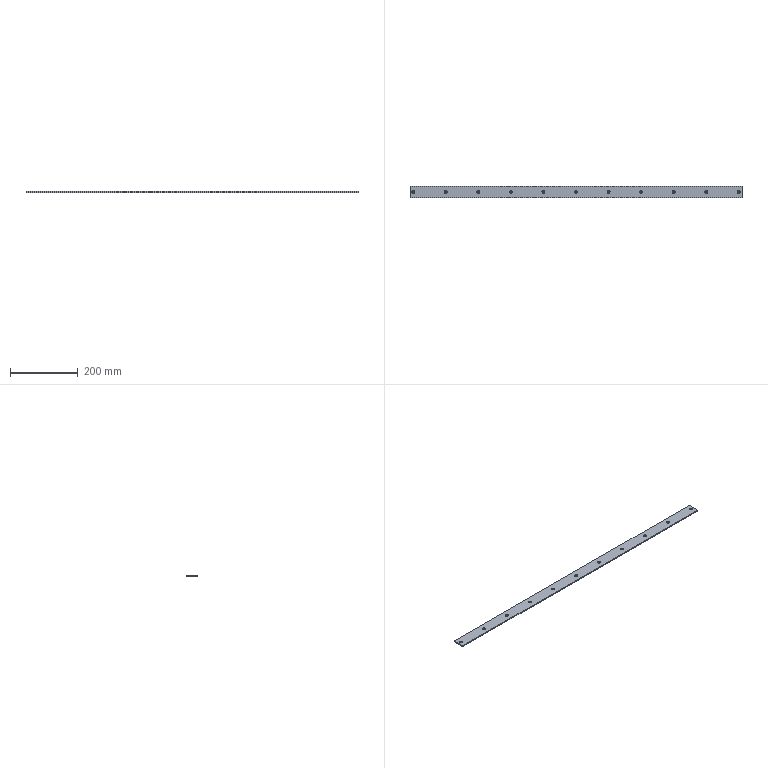Part | SolidWorks | features BaseBody 1 | 1 solid | 50 faces | box 979 x 35 x 3.2 mm | volume 108662 mm3 | cylinder 22 | cone 22 | plane 6 | commonest cylinder face diameters 4.5 x22
STEP:
#1=CARTESIAN_POINT('',(967.25,17.5,-3.2));
#2=VERTEX_POINT('',#1);
#3=CARTESIAN_POINT('',(971.75,17.5,-3.2));
#4=VERTEX_POINT('',#3);
#5=CARTESIAN_POINT('',(969.5,17.5,-3.2));
#6=DIRECTION('',(0.,0.,1.));
#7=DIRECTION('',(1.,0.,0.));
#8=AXIS2_PLACEMENT_3D('',#5,#6,#7);
#9=CIRCLE('',#8,2.25);
#10=EDGE_CURVE('',#2,#4,#9,.T.);
#11=ORIENTED_EDGE('',*,*,#10,.F.);
#12=CARTESIAN_POINT('',(967.25,17.5,-2.05));
#13=VERTEX_POINT('',#12);
#14=CARTESIAN_POINT('',(967.25,17.5,0.));
#15=DIRECTION('',(0.,0.,1.));
#16=VECTOR('',#15,1000.);
#17=LINE('',#14,#16);
#18=EDGE_CURVE('',#2,#13,#17,.T.);
#19=ORIENTED_EDGE('',*,*,#18,.T.);
#20=CARTESIAN_POINT('',(971.75,17.5,-2.05));
#21=VERTEX_POINT('',#20);
#22=CARTESIAN_POINT('',(969.5,17.5,-2.05));
#23=DIRECTION('',(0.,0.,-1.));
#24=DIRECTION('',(1.,0.,0.));
#25=AXIS2_PLACEMENT_3D('',#22,#23,#24);
#26=CIRCLE('',#25,2.25);
#27=EDGE_CURVE('',#21,#13,#26,.T.);
#28=ORIENTED_EDGE('',*,*,#27,.F.);
#29=CARTESIAN_POINT('',(971.75,17.5,0.));
#30=DIRECTION('',(0.,0.,1.));
#31=VECTOR('',#30,1000.);
#32=LINE('',#29,#31);
#33=EDGE_CURVE('',#4,#21,#32,.T.);
#34=ORIENTED_EDGE('',*,*,#33,.F.);
#35=EDGE_LOOP('',(#11,#19,#28,#34));
#36=FACE_OUTER_BOUND('',#35,.T.);
#37=CARTESIAN_POINT('',(969.5,17.5,0.));
#38=DIRECTION('',(0.,0.,1.));
#39=DIRECTION('',(1.,0.,0.));
#40=AXIS2_PLACEMENT_3D('',#37,#38,#39);
#41=CYLINDRICAL_SURFACE('',#40,2.25);
#42=ADVANCED_FACE('',(#36),#41,.F.);
#43=CARTESIAN_POINT('',(871.25,17.5,-3.2));
#44=VERTEX_POINT('',#43);
#45=CARTESIAN_POINT('',(875.75,17.5,-3.2));
#46=VERTEX_POINT('',#45);
#47=CARTESIAN_POINT('',(873.5,17.5,-3.2));
#48=DIRECTION('',(0.,0.,1.));
#49=DIRECTION('',(1.,0.,0.));
#50=AXIS2_PLACEMENT_3D('',#47,#48,#49);
#51=CIRCLE('',#50,2.25);
#52=EDGE_CURVE('',#44,#46,#51,.T.);
#53=ORIENTED_EDGE('',*,*,#52,.F.);
#54=CARTESIAN_POINT('',(871.25,17.5,-2.05));
#55=VERTEX_POINT('',#54);
#56=CARTESIAN_POINT('',(871.25,17.5,0.));
#57=DIRECTION('',(0.,0.,1.));
#58=VECTOR('',#57,1000.);
#59=LINE('',#56,#58);
#60=EDGE_CURVE('',#44,#55,#59,.T.);
#61=ORIENTED_EDGE('',*,*,#60,.T.);
#62=CARTESIAN_POINT('',(875.75,17.5,-2.05));
#63=VERTEX_POINT('',#62);
#64=CARTESIAN_POINT('',(873.5,17.5,-2.05));
#65=DIRECTION('',(0.,0.,-1.));
#66=DIRECTION('',(1.,0.,0.));
#67=AXIS2_PLACEMENT_3D('',#64,#65,#66);
#68=CIRCLE('',#67,2.25);
#69=EDGE_CURVE('',#63,#55,#68,.T.);
#70=ORIENTED_EDGE('',*,*,#69,.F.);
#71=CARTESIAN_POINT('',(875.75,17.5,0.));
#72=DIRECTION('',(0.,0.,1.));
#73=VECTOR('',#72,1000.);
#74=LINE('',#71,#73);
#75=EDGE_CURVE('',#46,#63,#74,.T.);
#76=ORIENTED_EDGE('',*,*,#75,.F.);
#77=EDGE_LOOP('',(#53,#61,#70,#76));
#78=FACE_OUTER_BOUND('',#77,.T.);
#79=CARTESIAN_POINT('',(873.5,17.5,0.));
#80=DIRECTION('',(0.,0.,1.));
#81=DIRECTION('',(1.,0.,0.));
#82=AXIS2_PLACEMENT_3D('',#79,#80,#81);
#83=CYLINDRICAL_SURFACE('',#82,2.25);
#84=ADVANCED_FACE('',(#78),#83,.F.);
#85=CARTESIAN_POINT('',(775.25,17.5,-3.2));
#86=VERTEX_POINT('',#85);
#87=CARTESIAN_POINT('',(779.75,17.5,-3.2));
#88=VERTEX_POINT('',#87);
#89=CARTESIAN_POINT('',(777.5,17.5,-3.2));
#90=DIRECTION('',(0.,0.,1.));
#91=DIRECTION('',(1.,0.,0.));
#92=AXIS2_PLACEMENT_3D('',#89,#90,#91);
#93=CIRCLE('',#92,2.25);
#94=EDGE_CURVE('',#86,#88,#93,.T.);
#95=ORIENTED_EDGE('',*,*,#94,.F.);
#96=CARTESIAN_POINT('',(775.25,17.5,-2.05));
#97=VERTEX_POINT('',#96);
#98=CARTESIAN_POINT('',(775.25,17.5,0.));
#99=DIRECTION('',(0.,0.,1.));
#100=VECTOR('',#99,1000.);
#101=LINE('',#98,#100);
#102=EDGE_CURVE('',#86,#97,#101,.T.);
#103=ORIENTED_EDGE('',*,*,#102,.T.);
#104=CARTESIAN_POINT('',(779.75,17.5,-2.05));
#105=VERTEX_POINT('',#104);
#106=CARTESIAN_POINT('',(777.5,17.5,-2.05));
#107=DIRECTION('',(0.,0.,-1.));
#108=DIRECTION('',(1.,0.,0.));
#109=AXIS2_PLACEMENT_3D('',#106,#107,#108);
#110=CIRCLE('',#109,2.25);
#111=EDGE_CURVE('',#105,#97,#110,.T.);
#112=ORIENTED_EDGE('',*,*,#111,.F.);
#113=CARTESIAN_POINT('',(779.75,17.5,0.));
#114=DIRECTION('',(0.,0.,1.));
#115=VECTOR('',#114,1000.);
#116=LINE('',#113,#115);
#117=EDGE_CURVE('',#88,#105,#116,.T.);
#118=ORIENTED_EDGE('',*,*,#117,.F.);
#119=EDGE_LOOP('',(#95,#103,#112,#118));
#120=FACE_OUTER_BOUND('',#119,.T.);
#121=CARTESIAN_POINT('',(777.5,17.5,0.));
#122=DIRECTION('',(0.,0.,1.));
#123=DIRECTION('',(1.,0.,0.));
#124=AXIS2_PLACEMENT_3D('',#121,#122,#123);
#125=CYLINDRICAL_SURFACE('',#124,2.25);
#126=ADVANCED_FACE('',(#120),#125,.F.);
#127=CARTESIAN_POINT('',(679.25,17.5,-3.2));
#128=VERTEX_POINT('',#127);
#129=CARTESIAN_POINT('',(683.75,17.5,-3.2));
#130=VERTEX_POINT('',#129);
#131=CARTESIAN_POINT('',(681.5,17.5,-3.2));
#132=DIRECTION('',(0.,0.,1.));
#133=DIRECTION('',(1.,0.,0.));
#134=AXIS2_PLACEMENT_3D('',#131,#132,#133);
#135=CIRCLE('',#134,2.25);
#136=EDGE_CURVE('',#128,#130,#135,.T.);
#137=ORIENTED_EDGE('',*,*,#136,.F.);
#138=CARTESIAN_POINT('',(679.25,17.5,-2.05));
#139=VERTEX_POINT('',#138);
#140=CARTESIAN_POINT('',(679.25,17.5,0.));
#141=DIRECTION('',(0.,0.,1.));
#142=VECTOR('',#141,1000.);
#143=LINE('',#140,#142);
#144=EDGE_CURVE('',#128,#139,#143,.T.);
#145=ORIENTED_EDGE('',*,*,#144,.T.);
#146=CARTESIAN_POINT('',(683.75,17.5,-2.05));
#147=VERTEX_POINT('',#146);
#148=CARTESIAN_POINT('',(681.5,17.5,-2.05));
#149=DIRECTION('',(0.,0.,-1.));
#150=DIRECTION('',(1.,0.,0.));
#151=AXIS2_PLACEMENT_3D('',#148,#149,#150);
#152=CIRCLE('',#151,2.25);
#153=EDGE_CURVE('',#147,#139,#152,.T.);
#154=ORIENTED_EDGE('',*,*,#153,.F.);
#155=CARTESIAN_POINT('',(683.75,17.5,0.));
#156=DIRECTION('',(0.,0.,1.));
#157=VECTOR('',#156,1000.);
#158=LINE('',#155,#157);
#159=EDGE_CURVE('',#130,#147,#158,.T.);
#160=ORIENTED_EDGE('',*,*,#159,.F.);
#161=EDGE_LOOP('',(#137,#145,#154,#160));
#162=FACE_OUTER_BOUND('',#161,.T.);
#163=CARTESIAN_POINT('',(681.5,17.5,0.));
#164=DIRECTION('',(0.,0.,1.));
#165=DIRECTION('',(1.,0.,0.));
#166=AXIS2_PLACEMENT_3D('',#163,#164,#165);
#167=CYLINDRICAL_SURFACE('',#166,2.25);
#168=ADVANCED_FACE('',(#162),#167,.F.);
#169=CARTESIAN_POINT('',(583.25,17.5,-3.2));
#170=VERTEX_POINT('',#169);
#171=CARTESIAN_POINT('',(587.75,17.5,-3.2));
#172=VERTEX_POINT('',#171);
#173=CARTESIAN_POINT('',(585.5,17.5,-3.2));
#174=DIRECTION('',(0.,0.,1.));
#175=DIRECTION('',(1.,0.,0.));
#176=AXIS2_PLACEMENT_3D('',#173,#174,#175);
#177=CIRCLE('',#176,2.25);
#178=EDGE_CURVE('',#170,#172,#177,.T.);
#179=ORIENTED_EDGE('',*,*,#178,.F.);
#180=CARTESIAN_POINT('',(583.25,17.5,-2.05));
#181=VERTEX_POINT('',#180);
#182=CARTESIAN_POINT('',(583.25,17.5,0.));
#183=DIRECTION('',(0.,0.,1.));
#184=VECTOR('',#183,1000.);
#185=LINE('',#182,#184);
#186=EDGE_CURVE('',#170,#181,#185,.T.);
#187=ORIENTED_EDGE('',*,*,#186,.T.);
#188=CARTESIAN_POINT('',(587.75,17.5,-2.05));
#189=VERTEX_POINT('',#188);
#190=CARTESIAN_POINT('',(585.5,17.5,-2.05));
#191=DIRECTION('',(0.,0.,-1.));
#192=DIRECTION('',(1.,0.,0.));
#193=AXIS2_PLACEMENT_3D('',#190,#191,#192);
#194=CIRCLE('',#193,2.25);
#195=EDGE_CURVE('',#189,#181,#194,.T.);
#196=ORIENTED_EDGE('',*,*,#195,.F.);
#197=CARTESIAN_POINT('',(587.75,17.5,0.));
#198=DIRECTION('',(0.,0.,1.));
#199=VECTOR('',#198,1000.);
#200=LINE('',#197,#199);
#201=EDGE_CURVE('',#172,#189,#200,.T.);
#202=ORIENTED_EDGE('',*,*,#201,.F.);
#203=EDGE_LOOP('',(#179,#187,#196,#202));
#204=FACE_OUTER_BOUND('',#203,.T.);
#205=CARTESIAN_POINT('',(585.5,17.5,0.));
#206=DIRECTION('',(0.,0.,1.));
#207=DIRECTION('',(1.,0.,0.));
#208=AXIS2_PLACEMENT_3D('',#205,#206,#207);
#209=CYLINDRICAL_SURFACE('',#208,2.25);
#210=ADVANCED_FACE('',(#204),#209,.F.);
#211=CARTESIAN_POINT('',(487.25,17.5,-3.2));
#212=VERTEX_POINT('',#211);
#213=CARTESIAN_POINT('',(491.75,17.5,-3.2));
#214=VERTEX_POINT('',#213);
#215=CARTESIAN_POINT('',(489.5,17.5,-3.2));
#216=DIRECTION('',(0.,0.,1.));
#217=DIRECTION('',(1.,0.,0.));
#218=AXIS2_PLACEMENT_3D('',#215,#216,#217);
#219=CIRCLE('',#218,2.25);
#220=EDGE_CURVE('',#212,#214,#219,.T.);
#221=ORIENTED_EDGE('',*,*,#220,.F.);
#222=CARTESIAN_POINT('',(487.25,17.5,-2.05));
#223=VERTEX_POINT('',#222);
#224=CARTESIAN_POINT('',(487.25,17.5,0.));
#225=DIRECTION('',(0.,0.,1.));
#226=VECTOR('',#225,1000.);
#227=LINE('',#224,#226);
#228=EDGE_CURVE('',#212,#223,#227,.T.);
#229=ORIENTED_EDGE('',*,*,#228,.T.);
#230=CARTESIAN_POINT('',(491.75,17.5,-2.05));
#231=VERTEX_POINT('',#230);
#232=CARTESIAN_POINT('',(489.5,17.5,-2.05));
#233=DIRECTION('',(0.,0.,-1.));
#234=DIRECTION('',(1.,0.,0.));
#235=AXIS2_PLACEMENT_3D('',#232,#233,#234);
#236=CIRCLE('',#235,2.25);
#237=EDGE_CURVE('',#231,#223,#236,.T.);
#238=ORIENTED_EDGE('',*,*,#237,.F.);
#239=CARTESIAN_POINT('',(491.75,17.5,0.));
#240=DIRECTION('',(0.,0.,1.));
#241=VECTOR('',#240,1000.);
#242=LINE('',#239,#241);
#243=EDGE_CURVE('',#214,#231,#242,.T.);
#244=ORIENTED_EDGE('',*,*,#243,.F.);
#245=EDGE_LOOP('',(#221,#229,#238,#244));
#246=FACE_OUTER_BOUND('',#245,.T.);
#247=CARTESIAN_POINT('',(489.5,17.5,0.));
#248=DIRECTION('',(0.,0.,1.));
#249=DIRECTION('',(1.,0.,0.));
#250=AXIS2_PLACEMENT_3D('',#247,#248,#249);
#251=CYLINDRICAL_SURFACE('',#250,2.25);
#252=ADVANCED_FACE('',(#246),#251,.F.);
#253=CARTESIAN_POINT('',(391.25,17.5,-3.2));
#254=VERTEX_POINT('',#253);
#255=CARTESIAN_POINT('',(395.75,17.5,-3.2));
#256=VERTEX_POINT('',#255);
#257=CARTESIAN_POINT('',(393.5,17.5,-3.2));
#258=DIRECTION('',(0.,0.,1.));
#259=DIRECTION('',(1.,0.,0.));
#260=AXIS2_PLACEMENT_3D('',#257,#258,#259);
#261=CIRCLE('',#260,2.25);
#262=EDGE_CURVE('',#254,#256,#261,.T.);
#263=ORIENTED_EDGE('',*,*,#262,.F.);
#264=CARTESIAN_POINT('',(391.25,17.5,-2.05));
#265=VERTEX_POINT('',#264);
#266=CARTESIAN_POINT('',(391.25,17.5,0.));
#267=DIRECTION('',(0.,0.,1.));
#268=VECTOR('',#267,1000.);
#269=LINE('',#266,#268);
#270=EDGE_CURVE('',#254,#265,#269,.T.);
#271=ORIENTED_EDGE('',*,*,#270,.T.);
#272=CARTESIAN_POINT('',(395.75,17.5,-2.05));
#273=VERTEX_POINT('',#272);
#274=CARTESIAN_POINT('',(393.5,17.5,-2.05));
#275=DIRECTION('',(0.,0.,-1.));
#276=DIRECTION('',(1.,0.,0.));
#277=AXIS2_PLACEMENT_3D('',#274,#275,#276);
#278=CIRCLE('',#277,2.25);
#279=EDGE_CURVE('',#273,#265,#278,.T.);
#280=ORIENTED_EDGE('',*,*,#279,.F.);
#281=CARTESIAN_POINT('',(395.75,17.5,0.));
#282=DIRECTION('',(0.,0.,1.));
#283=VECTOR('',#282,1000.);
#284=LINE('',#281,#283);
#285=EDGE_CURVE('',#256,#273,#284,.T.);
#286=ORIENTED_EDGE('',*,*,#285,.F.);
#287=EDGE_LOOP('',(#263,#271,#280,#286));
#288=FACE_OUTER_BOUND('',#287,.T.);
#289=CARTESIAN_POINT('',(393.5,17.5,0.));
#290=DIRECTION('',(0.,0.,1.));
#291=DIRECTION('',(1.,0.,0.));
#292=AXIS2_PLACEMENT_3D('',#289,#290,#291);
#293=CYLINDRICAL_SURFACE('',#292,2.25);
#294=ADVANCED_FACE('',(#288),#293,.F.);
#295=CARTESIAN_POINT('',(295.25,17.5,-3.2));
#296=VERTEX_POINT('',#295);
#297=CARTESIAN_POINT('',(299.75,17.5,-3.2));
#298=VERTEX_POINT('',#297);
#299=CARTESIAN_POINT('',(297.5,17.5,-3.2));
#300=DIRECTION('',(0.,0.,1.));
#301=DIRECTION('',(1.,0.,0.));
#302=AXIS2_PLACEMENT_3D('',#299,#300,#301);
#303=CIRCLE('',#302,2.25);
#304=EDGE_CURVE('',#296,#298,#303,.T.);
#305=ORIENTED_EDGE('',*,*,#304,.F.);
#306=CARTESIAN_POINT('',(295.25,17.5,-2.05));
#307=VERTEX_POINT('',#306);
#308=CARTESIAN_POINT('',(295.25,17.5,0.));
#309=DIRECTION('',(0.,0.,1.));
#310=VECTOR('',#309,1000.);
#311=LINE('',#308,#310);
#312=EDGE_CURVE('',#296,#307,#311,.T.);
#313=ORIENTED_EDGE('',*,*,#312,.T.);
#314=CARTESIAN_POINT('',(299.75,17.5,-2.05));
#315=VERTEX_POINT('',#314);
#316=CARTESIAN_POINT('',(297.5,17.5,-2.05));
#317=DIRECTION('',(0.,0.,-1.));
#318=DIRECTION('',(1.,0.,0.));
#319=AXIS2_PLACEMENT_3D('',#316,#317,#318);
#320=CIRCLE('',#319,2.25);
#321=EDGE_CURVE('',#315,#307,#320,.T.);
#322=ORIENTED_EDGE('',*,*,#321,.F.);
#323=CARTESIAN_POINT('',(299.75,17.5,0.));
#324=DIRECTION('',(0.,0.,1.));
#325=VECTOR('',#324,1000.);
#326=LINE('',#323,#325);
#327=EDGE_CURVE('',#298,#315,#326,.T.);
#328=ORIENTED_EDGE('',*,*,#327,.F.);
#329=EDGE_LOOP('',(#305,#313,#322,#328));
#330=FACE_OUTER_BOUND('',#329,.T.);
#331=CARTESIAN_POINT('',(297.5,17.5,0.));
#332=DIRECTION('',(0.,0.,1.));
#333=DIRECTION('',(1.,0.,0.));
#334=AXIS2_PLACEMENT_3D('',#331,#332,#333);
#335=CYLINDRICAL_SURFACE('',#334,2.25);
#336=ADVANCED_FACE('',(#330),#335,.F.);
#337=CARTESIAN_POINT('',(199.25,17.5,-3.2));
#338=VERTEX_POINT('',#337);
#339=CARTESIAN_POINT('',(203.75,17.5,-3.2));
#340=VERTEX_POINT('',#339);
#341=CARTESIAN_POINT('',(201.5,17.5,-3.2));
#342=DIRECTION('',(0.,0.,1.));
#343=DIRECTION('',(1.,0.,0.));
#344=AXIS2_PLACEMENT_3D('',#341,#342,#343);
#345=CIRCLE('',#344,2.25);
#346=EDGE_CURVE('',#338,#340,#345,.T.);
#347=ORIENTED_EDGE('',*,*,#346,.F.);
#348=CARTESIAN_POINT('',(199.25,17.5,-2.05));
#349=VERTEX_POINT('',#348);
#350=CARTESIAN_POINT('',(199.25,17.5,0.));
#351=DIRECTION('',(0.,0.,1.));
#352=VECTOR('',#351,1000.);
#353=LINE('',#350,#352);
#354=EDGE_CURVE('',#338,#349,#353,.T.);
#355=ORIENTED_EDGE('',*,*,#354,.T.);
#356=CARTESIAN_POINT('',(203.75,17.5,-2.05));
#357=VERTEX_POINT('',#356);
#358=CARTESIAN_POINT('',(201.5,17.5,-2.05));
#359=DIRECTION('',(0.,0.,-1.));
#360=DIRECTION('',(1.,0.,0.));
#361=AXIS2_PLACEMENT_3D('',#358,#359,#360);
#362=CIRCLE('',#361,2.25);
#363=EDGE_CURVE('',#357,#349,#362,.T.);
#364=ORIENTED_EDGE('',*,*,#363,.F.);
#365=CARTESIAN_POINT('',(203.75,17.5,0.));
#366=DIRECTION('',(0.,0.,1.));
#367=VECTOR('',#366,1000.);
#368=LINE('',#365,#367);
#369=EDGE_CURVE('',#340,#357,#368,.T.);
#370=ORIENTED_EDGE('',*,*,#369,.F.);
#371=EDGE_LOOP('',(#347,#355,#364,#370));
#372=FACE_OUTER_BOUND('',#371,.T.);
#373=CARTESIAN_POINT('',(201.5,17.5,0.));
#374=DIRECTION('',(0.,0.,1.));
#375=DIRECTION('',(1.,0.,0.));
#376=AXIS2_PLACEMENT_3D('',#373,#374,#375);
#377=CYLINDRICAL_SURFACE('',#376,2.25);
#378=ADVANCED_FACE('',(#372),#377,.F.);
#379=CARTESIAN_POINT('',(7.25,17.5,-3.2));
#380=VERTEX_POINT('',#379);
#381=CARTESIAN_POINT('',(11.75,17.5,-3.2));
#382=VERTEX_POINT('',#381);
#383=CARTESIAN_POINT('',(9.5,17.5,-3.2));
#384=DIRECTION('',(0.,0.,1.));
#385=DIRECTION('',(1.,0.,0.));
#386=AXIS2_PLACEMENT_3D('',#383,#384,#385);
#387=CIRCLE('',#386,2.25);
#388=EDGE_CURVE('',#380,#382,#387,.T.);
#389=ORIENTED_EDGE('',*,*,#388,.F.);
#390=CARTESIAN_POINT('',(7.25,17.5,-2.05));
#391=VERTEX_POINT('',#390);
#392=CARTESIAN_POINT('',(7.25,17.5,0.));
#393=DIRECTION('',(0.,0.,1.));
#394=VECTOR('',#393,1000.);
#395=LINE('',#392,#394);
#396=EDGE_CURVE('',#380,#391,#395,.T.);
#397=ORIENTED_EDGE('',*,*,#396,.T.);
#398=CARTESIAN_POINT('',(11.75,17.5,-2.05));
#399=VERTEX_POINT('',#398);
#400=CARTESIAN_POINT('',(9.5,17.5,-2.05));
#401=DIRECTION('',(0.,0.,-1.));
#402=DIRECTION('',(1.,0.,0.));
#403=AXIS2_PLACEMENT_3D('',#400,#401,#402);
#404=CIRCLE('',#403,2.25);
#405=EDGE_CURVE('',#399,#391,#404,.T.);
#406=ORIENTED_EDGE('',*,*,#405,.F.);
#407=CARTESIAN_POINT('',(11.75,17.5,0.));
#408=DIRECTION('',(0.,0.,1.));
#409=VECTOR('',#408,1000.);
#410=LINE('',#407,#409);
#411=EDGE_CURVE('',#382,#399,#410,.T.);
#412=ORIENTED_EDGE('',*,*,#411,.F.);
#413=EDGE_LOOP('',(#389,#397,#406,#412));
#414=FACE_OUTER_BOUND('',#413,.T.);
#415=CARTESIAN_POINT('',(9.5,17.5,0.));
#416=DIRECTION('',(0.,0.,1.));
#417=DIRECTION('',(1.,0.,0.));
#418=AXIS2_PLACEMENT_3D('',#415,#416,#417);
#419=CYLINDRICAL_SURFACE('',#418,2.25);
#420=ADVANCED_FACE('',(#414),#419,.F.);
#421=CARTESIAN_POINT('',(103.25,17.5,-3.2));
#422=VERTEX_POINT('',#421);
#423=CARTESIAN_POINT('',(107.75,17.5,-3.2));
#424=VERTEX_POINT('',#423);
#425=CARTESIAN_POINT('',(105.5,17.5,-3.2));
#426=DIRECTION('',(0.,0.,1.));
#427=DIRECTION('',(1.,0.,0.));
#428=AXIS2_PLACEMENT_3D('',#425,#426,#427);
#429=CIRCLE('',#428,2.25);
#430=EDGE_CURVE('',#422,#424,#429,.T.);
#431=ORIENTED_EDGE('',*,*,#430,.F.);
#432=CARTESIAN_POINT('',(103.25,17.5,-2.05));
#433=VERTEX_POINT('',#432);
#434=CARTESIAN_POINT('',(103.25,17.5,0.));
#435=DIRECTION('',(0.,0.,1.));
#436=VECTOR('',#435,1000.);
#437=LINE('',#434,#436);
#438=EDGE_CURVE('',#422,#433,#437,.T.);
#439=ORIENTED_EDGE('',*,*,#438,.T.);
#440=CARTESIAN_POINT('',(107.75,17.5,-2.05));
#441=VERTEX_POINT('',#440);
#442=CARTESIAN_POINT('',(105.5,17.5,-2.05));
#443=DIRECTION('',(0.,0.,-1.));
#444=DIRECTION('',(1.,0.,0.));
#445=AXIS2_PLACEMENT_3D('',#442,#443,#444);
#446=CIRCLE('',#445,2.25);
#447=EDGE_CURVE('',#441,#433,#446,.T.);
#448=ORIENTED_EDGE('',*,*,#447,.F.);
#449=CARTESIAN_POINT('',(107.75,17.5,0.));
#450=DIRECTION('',(0.,0.,1.));
#451=VECTOR('',#450,1000.);
#452=LINE('',#449,#451);
#453=EDGE_CURVE('',#424,#441,#452,.T.);
#454=ORIENTED_EDGE('',*,*,#453,.F.);
#455=EDGE_LOOP('',(#431,#439,#448,#454));
#456=FACE_OUTER_BOUND('',#455,.T.);
#457=CARTESIAN_POINT('',(105.5,17.5,0.));
#458=DIRECTION('',(0.,0.,1.));
#459=DIRECTION('',(1.,0.,0.));
#460=AXIS2_PLACEMENT_3D('',#457,#458,#459);
#461=CYLINDRICAL_SURFACE('',#460,2.25);
#462=ADVANCED_FACE('',(#456),#461,.F.);
#463=ORIENTED_EDGE('',*,*,#27,.T.);
#464=CARTESIAN_POINT('',(965.2,17.5,0.));
#465=VERTEX_POINT('',#464);
#466=CARTESIAN_POINT('',(965.2,17.5,0.));
#467=DIRECTION('',(-0.7071,0.,0.7071));
#468=VECTOR('',#467,1000.);
#469=LINE('',#466,#468);
#470=EDGE_CURVE('',#13,#465,#469,.T.);
#471=ORIENTED_EDGE('',*,*,#470,.T.);
#472=CARTESIAN_POINT('',(973.8,17.5,0.));
#473=VERTEX_POINT('',#472);
#474=CARTESIAN_POINT('',(969.5,17.5,0.));
#475=DIRECTION('',(0.,0.,-1.));
#476=DIRECTION('',(1.,0.,0.));
#477=AXIS2_PLACEMENT_3D('',#474,#475,#476);
#478=CIRCLE('',#477,4.3);
#479=EDGE_CURVE('',#473,#465,#478,.T.);
#480=ORIENTED_EDGE('',*,*,#479,.F.);
#481=CARTESIAN_POINT('',(973.8,17.5,0.));
#482=DIRECTION('',(0.7071,0.,0.7071));
#483=VECTOR('',#482,1000.);
#484=LINE('',#481,#483);
#485=EDGE_CURVE('',#21,#473,#484,.T.);
#486=ORIENTED_EDGE('',*,*,#485,.F.);
#487=EDGE_LOOP('',(#463,#471,#480,#486));
#488=FACE_OUTER_BOUND('',#487,.T.);
#489=CARTESIAN_POINT('',(969.5,17.5,0.));
#490=DIRECTION('',(0.,0.,1.));
#491=DIRECTION('',(1.,0.,0.));
#492=AXIS2_PLACEMENT_3D('',#489,#490,#491);
#493=CONICAL_SURFACE('',#492,4.3,0.7854);
#494=ADVANCED_FACE('',(#488),#493,.F.);
#495=ORIENTED_EDGE('',*,*,#69,.T.);
#496=CARTESIAN_POINT('',(869.2,17.5,0.));
#497=VERTEX_POINT('',#496);
#498=CARTESIAN_POINT('',(869.2,17.5,0.));
#499=DIRECTION('',(-0.7071,0.,0.7071));
#500=VECTOR('',#499,1000.);
#501=LINE('',#498,#500);
#502=EDGE_CURVE('',#55,#497,#501,.T.);
#503=ORIENTED_EDGE('',*,*,#502,.T.);
#504=CARTESIAN_POINT('',(877.8,17.5,0.));
#505=VERTEX_POINT('',#504);
#506=CARTESIAN_POINT('',(873.5,17.5,0.));
#507=DIRECTION('',(0.,0.,-1.));
#508=DIRECTION('',(1.,0.,0.));
#509=AXIS2_PLACEMENT_3D('',#506,#507,#508);
#510=CIRCLE('',#509,4.3);
#511=EDGE_CURVE('',#505,#497,#510,.T.);
#512=ORIENTED_EDGE('',*,*,#511,.F.);
#513=CARTESIAN_POINT('',(877.8,17.5,0.));
#514=DIRECTION('',(0.7071,0.,0.7071));
#515=VECTOR('',#514,1000.);
#516=LINE('',#513,#515);
#517=EDGE_CURVE('',#63,#505,#516,.T.);
#518=ORIENTED_EDGE('',*,*,#517,.F.);
#519=EDGE_LOOP('',(#495,#503,#512,#518));
#520=FACE_OUTER_BOUND('',#519,.T.);
#521=CARTESIAN_POINT('',(873.5,17.5,0.));
#522=DIRECTION('',(0.,0.,1.));
#523=DIRECTION('',(1.,0.,0.));
#524=AXIS2_PLACEMENT_3D('',#521,#522,#523);
#525=CONICAL_SURFACE('',#524,4.3,0.7854);
#526=ADVANCED_FACE('',(#520),#525,.F.);
#527=ORIENTED_EDGE('',*,*,#111,.T.);
#528=CARTESIAN_POINT('',(773.2,17.5,0.));
#529=VERTEX_POINT('',#528);
#530=CARTESIAN_POINT('',(773.2,17.5,0.));
#531=DIRECTION('',(-0.7071,0.,0.7071));
#532=VECTOR('',#531,1000.);
#533=LINE('',#530,#532);
#534=EDGE_CURVE('',#97,#529,#533,.T.);
#535=ORIENTED_EDGE('',*,*,#534,.T.);
#536=CARTESIAN_POINT('',(781.8,17.5,0.));
#537=VERTEX_POINT('',#536);
#538=CARTESIAN_POINT('',(777.5,17.5,0.));
#539=DIRECTION('',(0.,0.,-1.));
#540=DIRECTION('',(1.,0.,0.));
#541=AXIS2_PLACEMENT_3D('',#538,#539,#540);
#542=CIRCLE('',#541,4.3);
#543=EDGE_CURVE('',#537,#529,#542,.T.);
#544=ORIENTED_EDGE('',*,*,#543,.F.);
#545=CARTESIAN_POINT('',(781.8,17.5,0.));
#546=DIRECTION('',(0.7071,0.,0.7071));
#547=VECTOR('',#546,1000.);
#548=LINE('',#545,#547);
#549=EDGE_CURVE('',#105,#537,#548,.T.);
#550=ORIENTED_EDGE('',*,*,#549,.F.);
#551=EDGE_LOOP('',(#527,#535,#544,#550));
#552=FACE_OUTER_BOUND('',#551,.T.);
#553=CARTESIAN_POINT('',(777.5,17.5,0.));
#554=DIRECTION('',(0.,0.,1.));
#555=DIRECTION('',(1.,0.,0.));
#556=AXIS2_PLACEMENT_3D('',#553,#554,#555);
#557=CONICAL_SURFACE('',#556,4.3,0.7854);
#558=ADVANCED_FACE('',(#552),#557,.F.);
#559=ORIENTED_EDGE('',*,*,#153,.T.);
#560=CARTESIAN_POINT('',(677.2,17.5,0.));
#561=VERTEX_POINT('',#560);
#562=CARTESIAN_POINT('',(677.2,17.5,0.));
#563=DIRECTION('',(-0.7071,0.,0.7071));
#564=VECTOR('',#563,1000.);
#565=LINE('',#562,#564);
#566=EDGE_CURVE('',#139,#561,#565,.T.);
#567=ORIENTED_EDGE('',*,*,#566,.T.);
#568=CARTESIAN_POINT('',(685.8,17.5,0.));
#569=VERTEX_POINT('',#568);
#570=CARTESIAN_POINT('',(681.5,17.5,0.));
#571=DIRECTION('',(0.,0.,-1.));
#572=DIRECTION('',(1.,0.,0.));
#573=AXIS2_PLACEMENT_3D('',#570,#571,#572);
#574=CIRCLE('',#573,4.3);
#575=EDGE_CURVE('',#569,#561,#574,.T.);
#576=ORIENTED_EDGE('',*,*,#575,.F.);
#577=CARTESIAN_POINT('',(685.8,17.5,0.));
#578=DIRECTION('',(0.7071,0.,0.7071));
#579=VECTOR('',#578,1000.);
#580=LINE('',#577,#579);
#581=EDGE_CURVE('',#147,#569,#580,.T.);
#582=ORIENTED_EDGE('',*,*,#581,.F.);
#583=EDGE_LOOP('',(#559,#567,#576,#582));
#584=FACE_OUTER_BOUND('',#583,.T.);
#585=CARTESIAN_POINT('',(681.5,17.5,0.));
#586=DIRECTION('',(0.,0.,1.));
#587=DIRECTION('',(1.,0.,0.));
#588=AXIS2_PLACEMENT_3D('',#585,#586,#587);
#589=CONICAL_SURFACE('',#588,4.3,0.7854);
#590=ADVANCED_FACE('',(#584),#589,.F.);
#591=ORIENTED_EDGE('',*,*,#195,.T.);
#592=CARTESIAN_POINT('',(581.2,17.5,0.));
#593=VERTEX_POINT('',#592);
#594=CARTESIAN_POINT('',(581.2,17.5,0.));
#595=DIRECTION('',(-0.7071,0.,0.7071));
#596=VECTOR('',#595,1000.);
#597=LINE('',#594,#596);
#598=EDGE_CURVE('',#181,#593,#597,.T.);
#599=ORIENTED_EDGE('',*,*,#598,.T.);
#600=CARTESIAN_POINT('',(589.8,17.5,0.));
#601=VERTEX_POINT('',#600);
#602=CARTESIAN_POINT('',(585.5,17.5,0.));
#603=DIRECTION('',(0.,0.,-1.));
#604=DIRECTION('',(1.,0.,0.));
#605=AXIS2_PLACEMENT_3D('',#602,#603,#604);
#606=CIRCLE('',#605,4.3);
#607=EDGE_CURVE('',#601,#593,#606,.T.);
#608=ORIENTED_EDGE('',*,*,#607,.F.);
#609=CARTESIAN_POINT('',(589.8,17.5,0.));
#610=DIRECTION('',(0.7071,0.,0.7071));
#611=VECTOR('',#610,1000.);
#612=LINE('',#609,#611);
#613=EDGE_CURVE('',#189,#601,#612,.T.);
#614=ORIENTED_EDGE('',*,*,#613,.F.);
#615=EDGE_LOOP('',(#591,#599,#608,#614));
#616=FACE_OUTER_BOUND('',#615,.T.);
#617=CARTESIAN_POINT('',(585.5,17.5,0.));
#618=DIRECTION('',(0.,0.,1.));
#619=DIRECTION('',(1.,0.,0.));
#620=AXIS2_PLACEMENT_3D('',#617,#618,#619);
#621=CONICAL_SURFACE('',#620,4.3,0.7854);
#622=ADVANCED_FACE('',(#616),#621,.F.);
#623=ORIENTED_EDGE('',*,*,#237,.T.);
#624=CARTESIAN_POINT('',(485.2,17.5,0.));
#625=VERTEX_POINT('',#624);
#626=CARTESIAN_POINT('',(485.2,17.5,0.));
#627=DIRECTION('',(-0.7071,0.,0.7071));
#628=VECTOR('',#627,1000.);
#629=LINE('',#626,#628);
#630=EDGE_CURVE('',#223,#625,#629,.T.);
#631=ORIENTED_EDGE('',*,*,#630,.T.);
#632=CARTESIAN_POINT('',(493.8,17.5,0.));
#633=VERTEX_POINT('',#632);
#634=CARTESIAN_POINT('',(489.5,17.5,0.));
#635=DIRECTION('',(0.,0.,-1.));
#636=DIRECTION('',(1.,0.,0.));
#637=AXIS2_PLACEMENT_3D('',#634,#635,#636);
#638=CIRCLE('',#637,4.3);
#639=EDGE_CURVE('',#633,#625,#638,.T.);
#640=ORIENTED_EDGE('',*,*,#639,.F.);
#641=CARTESIAN_POINT('',(493.8,17.5,0.));
#642=DIRECTION('',(0.7071,0.,0.7071));
#643=VECTOR('',#642,1000.);
#644=LINE('',#641,#643);
#645=EDGE_CURVE('',#231,#633,#644,.T.);
#646=ORIENTED_EDGE('',*,*,#645,.F.);
#647=EDGE_LOOP('',(#623,#631,#640,#646));
#648=FACE_OUTER_BOUND('',#647,.T.);
#649=CARTESIAN_POINT('',(489.5,17.5,0.));
#650=DIRECTION('',(0.,0.,1.));
#651=DIRECTION('',(1.,0.,0.));
#652=AXIS2_PLACEMENT_3D('',#649,#650,#651);
#653=CONICAL_SURFACE('',#652,4.3,0.7854);
#654=ADVANCED_FACE('',(#648),#653,.F.);
#655=ORIENTED_EDGE('',*,*,#279,.T.);
#656=CARTESIAN_POINT('',(389.2,17.5,0.));
#657=VERTEX_POINT('',#656);
#658=CARTESIAN_POINT('',(389.2,17.5,0.));
#659=DIRECTION('',(-0.7071,0.,0.7071));
#660=VECTOR('',#659,1000.);
#661=LINE('',#658,#660);
#662=EDGE_CURVE('',#265,#657,#661,.T.);
#663=ORIENTED_EDGE('',*,*,#662,.T.);
#664=CARTESIAN_POINT('',(397.8,17.5,0.));
#665=VERTEX_POINT('',#664);
#666=CARTESIAN_POINT('',(393.5,17.5,0.));
#667=DIRECTION('',(0.,0.,-1.));
#668=DIRECTION('',(1.,0.,0.));
#669=AXIS2_PLACEMENT_3D('',#666,#667,#668);
#670=CIRCLE('',#669,4.3);
#671=EDGE_CURVE('',#665,#657,#670,.T.);
#672=ORIENTED_EDGE('',*,*,#671,.F.);
#673=CARTESIAN_POINT('',(397.8,17.5,0.));
#674=DIRECTION('',(0.7071,0.,0.7071));
#675=VECTOR('',#674,1000.);
#676=LINE('',#673,#675);
#677=EDGE_CURVE('',#273,#665,#676,.T.);
#678=ORIENTED_EDGE('',*,*,#677,.F.);
#679=EDGE_LOOP('',(#655,#663,#672,#678));
#680=FACE_OUTER_BOUND('',#679,.T.);
#681=CARTESIAN_POINT('',(393.5,17.5,0.));
#682=DIRECTION('',(0.,0.,1.));
#683=DIRECTION('',(1.,0.,0.));
#684=AXIS2_PLACEMENT_3D('',#681,#682,#683);
#685=CONICAL_SURFACE('',#684,4.3,0.7854);
#686=ADVANCED_FACE('',(#680),#685,.F.);
#687=ORIENTED_EDGE('',*,*,#321,.T.);
#688=CARTESIAN_POINT('',(293.2,17.5,0.));
#689=VERTEX_POINT('',#688);
#690=CARTESIAN_POINT('',(293.2,17.5,0.));
#691=DIRECTION('',(-0.7071,0.,0.7071));
#692=VECTOR('',#691,1000.);
#693=LINE('',#690,#692);
#694=EDGE_CURVE('',#307,#689,#693,.T.);
#695=ORIENTED_EDGE('',*,*,#694,.T.);
#696=CARTESIAN_POINT('',(301.8,17.5,0.));
#697=VERTEX_POINT('',#696);
#698=CARTESIAN_POINT('',(297.5,17.5,0.));
#699=DIRECTION('',(0.,0.,-1.));
#700=DIRECTION('',(1.,0.,0.));
#701=AXIS2_PLACEMENT_3D('',#698,#699,#700);
#702=CIRCLE('',#701,4.3);
#703=EDGE_CURVE('',#697,#689,#702,.T.);
#704=ORIENTED_EDGE('',*,*,#703,.F.);
#705=CARTESIAN_POINT('',(301.8,17.5,0.));
#706=DIRECTION('',(0.7071,0.,0.7071));
#707=VECTOR('',#706,1000.);
#708=LINE('',#705,#707);
#709=EDGE_CURVE('',#315,#697,#708,.T.);
#710=ORIENTED_EDGE('',*,*,#709,.F.);
#711=EDGE_LOOP('',(#687,#695,#704,#710));
#712=FACE_OUTER_BOUND('',#711,.T.);
#713=CARTESIAN_POINT('',(297.5,17.5,0.));
#714=DIRECTION('',(0.,0.,1.));
#715=DIRECTION('',(1.,0.,0.));
#716=AXIS2_PLACEMENT_3D('',#713,#714,#715);
#717=CONICAL_SURFACE('',#716,4.3,0.7854);
#718=ADVANCED_FACE('',(#712),#717,.F.);
#719=ORIENTED_EDGE('',*,*,#363,.T.);
#720=CARTESIAN_POINT('',(197.2,17.5,0.));
#721=VERTEX_POINT('',#720);
#722=CARTESIAN_POINT('',(197.2,17.5,0.));
#723=DIRECTION('',(-0.7071,0.,0.7071));
#724=VECTOR('',#723,1000.);
#725=LINE('',#722,#724);
#726=EDGE_CURVE('',#349,#721,#725,.T.);
#727=ORIENTED_EDGE('',*,*,#726,.T.);
#728=CARTESIAN_POINT('',(205.8,17.5,0.));
#729=VERTEX_POINT('',#728);
#730=CARTESIAN_POINT('',(201.5,17.5,0.));
#731=DIRECTION('',(0.,0.,-1.));
#732=DIRECTION('',(1.,0.,0.));
#733=AXIS2_PLACEMENT_3D('',#730,#731,#732);
#734=CIRCLE('',#733,4.3);
#735=EDGE_CURVE('',#729,#721,#734,.T.);
#736=ORIENTED_EDGE('',*,*,#735,.F.);
#737=CARTESIAN_POINT('',(205.8,17.5,0.));
#738=DIRECTION('',(0.7071,0.,0.7071));
#739=VECTOR('',#738,1000.);
#740=LINE('',#737,#739);
#741=EDGE_CURVE('',#357,#729,#740,.T.);
#742=ORIENTED_EDGE('',*,*,#741,.F.);
#743=EDGE_LOOP('',(#719,#727,#736,#742));
#744=FACE_OUTER_BOUND('',#743,.T.);
#745=CARTESIAN_POINT('',(201.5,17.5,0.));
#746=DIRECTION('',(0.,0.,1.));
#747=DIRECTION('',(1.,0.,0.));
#748=AXIS2_PLACEMENT_3D('',#745,#746,#747);
#749=CONICAL_SURFACE('',#748,4.3,0.7854);
#750=ADVANCED_FACE('',(#744),#749,.F.);
#751=ORIENTED_EDGE('',*,*,#405,.T.);
#752=CARTESIAN_POINT('',(5.2,17.5,0.));
#753=VERTEX_POINT('',#752);
#754=CARTESIAN_POINT('',(5.2,17.5,0.));
#755=DIRECTION('',(-0.7071,0.,0.7071));
#756=VECTOR('',#755,1000.);
#757=LINE('',#754,#756);
#758=EDGE_CURVE('',#391,#753,#757,.T.);
#759=ORIENTED_EDGE('',*,*,#758,.T.);
#760=CARTESIAN_POINT('',(13.8,17.5,0.));
#761=VERTEX_POINT('',#760);
#762=CARTESIAN_POINT('',(9.5,17.5,0.));
#763=DIRECTION('',(0.,0.,1.));
#764=DIRECTION('',(1.,0.,0.));
#765=AXIS2_PLACEMENT_3D('',#762,#763,#764);
#766=CIRCLE('',#765,4.3);
#767=EDGE_CURVE('',#753,#761,#766,.T.);
#768=ORIENTED_EDGE('',*,*,#767,.T.);
#769=CARTESIAN_POINT('',(13.8,17.5,0.));
#770=DIRECTION('',(0.7071,0.,0.7071));
#771=VECTOR('',#770,1000.);
#772=LINE('',#769,#771);
#773=EDGE_CURVE('',#399,#761,#772,.T.);
#774=ORIENTED_EDGE('',*,*,#773,.F.);
#775=EDGE_LOOP('',(#751,#759,#768,#774));
#776=FACE_OUTER_BOUND('',#775,.T.);
#777=CARTESIAN_POINT('',(9.5,17.5,0.));
#778=DIRECTION('',(0.,0.,1.));
#779=DIRECTION('',(1.,0.,0.));
#780=AXIS2_PLACEMENT_3D('',#777,#778,#779);
#781=CONICAL_SURFACE('',#780,4.3,0.7854);
#782=ADVANCED_FACE('',(#776),#781,.F.);
#783=ORIENTED_EDGE('',*,*,#447,.T.);
#784=CARTESIAN_POINT('',(101.2,17.5,0.));
#785=VERTEX_POINT('',#784);
#786=CARTESIAN_POINT('',(101.2,17.5,0.));
#787=DIRECTION('',(-0.7071,0.,0.7071));
#788=VECTOR('',#787,1000.);
#789=LINE('',#786,#788);
#790=EDGE_CURVE('',#433,#785,#789,.T.);
#791=ORIENTED_EDGE('',*,*,#790,.T.);
#792=CARTESIAN_POINT('',(109.8,17.5,0.));
#793=VERTEX_POINT('',#792);
#794=CARTESIAN_POINT('',(105.5,17.5,0.));
#795=DIRECTION('',(0.,0.,1.));
#796=DIRECTION('',(1.,0.,0.));
#797=AXIS2_PLACEMENT_3D('',#794,#795,#796);
#798=CIRCLE('',#797,4.3);
#799=EDGE_CURVE('',#785,#793,#798,.T.);
#800=ORIENTED_EDGE('',*,*,#799,.T.);
#801=CARTESIAN_POINT('',(109.8,17.5,0.));
#802=DIRECTION('',(0.7071,0.,0.7071));
#803=VECTOR('',#802,1000.);
#804=LINE('',#801,#803);
#805=EDGE_CURVE('',#441,#793,#804,.T.);
#806=ORIENTED_EDGE('',*,*,#805,.F.);
#807=EDGE_LOOP('',(#783,#791,#800,#806));
#808=FACE_OUTER_BOUND('',#807,.T.);
#809=CARTESIAN_POINT('',(105.5,17.5,0.));
#810=DIRECTION('',(0.,0.,1.));
#811=DIRECTION('',(1.,0.,0.));
#812=AXIS2_PLACEMENT_3D('',#809,#810,#811);
#813=CONICAL_SURFACE('',#812,4.3,0.7854);
#814=ADVANCED_FACE('',(#808),#813,.F.);
#815=CARTESIAN_POINT('',(969.5,17.5,-3.2));
#816=DIRECTION('',(0.,0.,1.));
#817=DIRECTION('',(1.,0.,0.));
#818=AXIS2_PLACEMENT_3D('',#815,#816,#817);
#819=CIRCLE('',#818,2.25);
#820=EDGE_CURVE('',#4,#2,#819,.T.);
#821=ORIENTED_EDGE('',*,*,#820,.T.);
#822=ORIENTED_EDGE('',*,*,#10,.T.);
#823=EDGE_LOOP('',(#821,#822));
#824=FACE_BOUND('',#823,.T.);
#825=CARTESIAN_POINT('',(873.5,17.5,-3.2));
#826=DIRECTION('',(0.,0.,1.));
#827=DIRECTION('',(1.,0.,0.));
#828=AXIS2_PLACEMENT_3D('',#825,#826,#827);
#829=CIRCLE('',#828,2.25);
#830=EDGE_CURVE('',#46,#44,#829,.T.);
#831=ORIENTED_EDGE('',*,*,#830,.T.);
#832=ORIENTED_EDGE('',*,*,#52,.T.);
#833=EDGE_LOOP('',(#831,#832));
#834=FACE_BOUND('',#833,.T.);
#835=CARTESIAN_POINT('',(777.5,17.5,-3.2));
#836=DIRECTION('',(0.,0.,1.));
#837=DIRECTION('',(1.,0.,0.));
#838=AXIS2_PLACEMENT_3D('',#835,#836,#837);
#839=CIRCLE('',#838,2.25);
#840=EDGE_CURVE('',#88,#86,#839,.T.);
#841=ORIENTED_EDGE('',*,*,#840,.T.);
#842=ORIENTED_EDGE('',*,*,#94,.T.);
#843=EDGE_LOOP('',(#841,#842));
#844=FACE_BOUND('',#843,.T.);
#845=CARTESIAN_POINT('',(681.5,17.5,-3.2));
#846=DIRECTION('',(0.,0.,1.));
#847=DIRECTION('',(1.,0.,0.));
#848=AXIS2_PLACEMENT_3D('',#845,#846,#847);
#849=CIRCLE('',#848,2.25);
#850=EDGE_CURVE('',#130,#128,#849,.T.);
#851=ORIENTED_EDGE('',*,*,#850,.T.);
#852=ORIENTED_EDGE('',*,*,#136,.T.);
#853=EDGE_LOOP('',(#851,#852));
#854=FACE_BOUND('',#853,.T.);
#855=CARTESIAN_POINT('',(585.5,17.5,-3.2));
#856=DIRECTION('',(0.,0.,1.));
#857=DIRECTION('',(1.,0.,0.));
#858=AXIS2_PLACEMENT_3D('',#855,#856,#857);
#859=CIRCLE('',#858,2.25);
#860=EDGE_CURVE('',#172,#170,#859,.T.);
#861=ORIENTED_EDGE('',*,*,#860,.T.);
#862=ORIENTED_EDGE('',*,*,#178,.T.);
#863=EDGE_LOOP('',(#861,#862));
#864=FACE_BOUND('',#863,.T.);
#865=CARTESIAN_POINT('',(489.5,17.5,-3.2));
#866=DIRECTION('',(0.,0.,1.));
#867=DIRECTION('',(1.,0.,0.));
#868=AXIS2_PLACEMENT_3D('',#865,#866,#867);
#869=CIRCLE('',#868,2.25);
#870=EDGE_CURVE('',#214,#212,#869,.T.);
#871=ORIENTED_EDGE('',*,*,#870,.T.);
#872=ORIENTED_EDGE('',*,*,#220,.T.);
#873=EDGE_LOOP('',(#871,#872));
#874=FACE_BOUND('',#873,.T.);
#875=CARTESIAN_POINT('',(393.5,17.5,-3.2));
#876=DIRECTION('',(0.,0.,1.));
#877=DIRECTION('',(1.,0.,0.));
#878=AXIS2_PLACEMENT_3D('',#875,#876,#877);
#879=CIRCLE('',#878,2.25);
#880=EDGE_CURVE('',#256,#254,#879,.T.);
#881=ORIENTED_EDGE('',*,*,#880,.T.);
#882=ORIENTED_EDGE('',*,*,#262,.T.);
#883=EDGE_LOOP('',(#881,#882));
#884=FACE_BOUND('',#883,.T.);
#885=CARTESIAN_POINT('',(297.5,17.5,-3.2));
#886=DIRECTION('',(0.,0.,1.));
#887=DIRECTION('',(1.,0.,0.));
#888=AXIS2_PLACEMENT_3D('',#885,#886,#887);
#889=CIRCLE('',#888,2.25);
#890=EDGE_CURVE('',#298,#296,#889,.T.);
#891=ORIENTED_EDGE('',*,*,#890,.T.);
#892=ORIENTED_EDGE('',*,*,#304,.T.);
#893=EDGE_LOOP('',(#891,#892));
#894=FACE_BOUND('',#893,.T.);
#895=CARTESIAN_POINT('',(201.5,17.5,-3.2));
#896=DIRECTION('',(0.,0.,1.));
#897=DIRECTION('',(1.,0.,0.));
#898=AXIS2_PLACEMENT_3D('',#895,#896,#897);
#899=CIRCLE('',#898,2.25);
#900=EDGE_CURVE('',#340,#338,#899,.T.);
#901=ORIENTED_EDGE('',*,*,#900,.T.);
#902=ORIENTED_EDGE('',*,*,#346,.T.);
#903=EDGE_LOOP('',(#901,#902));
#904=FACE_BOUND('',#903,.T.);
#905=CARTESIAN_POINT('',(979.,35.,-3.2));
#906=VERTEX_POINT('',#905);
#907=CARTESIAN_POINT('',(979.,0.,-3.2));
#908=VERTEX_POINT('',#907);
#909=CARTESIAN_POINT('',(979.,0.,-3.2));
#910=DIRECTION('',(0.,-1.,0.));
#911=VECTOR('',#910,1000.);
#912=LINE('',#909,#911);
#913=EDGE_CURVE('',#906,#908,#912,.T.);
#914=ORIENTED_EDGE('',*,*,#913,.T.);
#915=CARTESIAN_POINT('',(0.,0.,-3.2));
#916=VERTEX_POINT('',#915);
#917=CARTESIAN_POINT('',(0.,0.,-3.2));
#918=DIRECTION('',(-1.,0.,0.));
#919=VECTOR('',#918,1000.);
#920=LINE('',#917,#919);
#921=EDGE_CURVE('',#908,#916,#920,.T.);
#922=ORIENTED_EDGE('',*,*,#921,.T.);
#923=CARTESIAN_POINT('',(0.,35.,-3.2));
#924=VERTEX_POINT('',#923);
#925=CARTESIAN_POINT('',(0.,0.,-3.2));
#926=DIRECTION('',(0.,1.,0.));
#927=VECTOR('',#926,1000.);
#928=LINE('',#925,#927);
#929=EDGE_CURVE('',#916,#924,#928,.T.);
#930=ORIENTED_EDGE('',*,*,#929,.T.);
#931=CARTESIAN_POINT('',(0.,35.,-3.2));
#932=DIRECTION('',(1.,0.,0.));
#933=VECTOR('',#932,1000.);
#934=LINE('',#931,#933);
#935=EDGE_CURVE('',#924,#906,#934,.T.);
#936=ORIENTED_EDGE('',*,*,#935,.T.);
#937=EDGE_LOOP('',(#914,#922,#930,#936));
#938=FACE_OUTER_BOUND('',#937,.T.);
#939=CARTESIAN_POINT('',(9.5,17.5,-3.2));
#940=DIRECTION('',(0.,0.,1.));
#941=DIRECTION('',(1.,0.,0.));
#942=AXIS2_PLACEMENT_3D('',#939,#940,#941);
#943=CIRCLE('',#942,2.25);
#944=EDGE_CURVE('',#382,#380,#943,.T.);
#945=ORIENTED_EDGE('',*,*,#944,.T.);
#946=ORIENTED_EDGE('',*,*,#388,.T.);
#947=EDGE_LOOP('',(#945,#946));
#948=FACE_BOUND('',#947,.T.);
#949=CARTESIAN_POINT('',(105.5,17.5,-3.2));
#950=DIRECTION('',(0.,0.,1.));
#951=DIRECTION('',(1.,0.,0.));
#952=AXIS2_PLACEMENT_3D('',#949,#950,#951);
#953=CIRCLE('',#952,2.25);
#954=EDGE_CURVE('',#424,#422,#953,.T.);
#955=ORIENTED_EDGE('',*,*,#954,.T.);
#956=ORIENTED_EDGE('',*,*,#430,.T.);
#957=EDGE_LOOP('',(#955,#956));
#958=FACE_BOUND('',#957,.T.);
#959=CARTESIAN_POINT('',(0.,0.,-3.2));
#960=DIRECTION('',(0.,0.,-1.));
#961=DIRECTION('',(-1.,0.,0.));
#962=AXIS2_PLACEMENT_3D('',#959,#960,#961);
#963=PLANE('',#962);
#964=ADVANCED_FACE('',(#824,#834,#844,#854,#864,#874,#884,#894,#904,#938,#948,#958),#963,.T.);
#965=ORIENTED_EDGE('',*,*,#18,.F.);
#966=ORIENTED_EDGE('',*,*,#820,.F.);
#967=ORIENTED_EDGE('',*,*,#33,.T.);
#968=CARTESIAN_POINT('',(969.5,17.5,-2.05));
#969=DIRECTION('',(0.,0.,-1.));
#970=DIRECTION('',(1.,0.,0.));
#971=AXIS2_PLACEMENT_3D('',#968,#969,#970);
#972=CIRCLE('',#971,2.25);
#973=EDGE_CURVE('',#13,#21,#972,.T.);
#974=ORIENTED_EDGE('',*,*,#973,.F.);
#975=EDGE_LOOP('',(#965,#966,#967,#974));
#976=FACE_OUTER_BOUND('',#975,.T.);
#977=CARTESIAN_POINT('',(969.5,17.5,0.));
#978=DIRECTION('',(0.,0.,1.));
#979=DIRECTION('',(1.,0.,0.));
#980=AXIS2_PLACEMENT_3D('',#977,#978,#979);
#981=CYLINDRICAL_SURFACE('',#980,2.25);
#982=ADVANCED_FACE('',(#976),#981,.F.);
#983=ORIENTED_EDGE('',*,*,#60,.F.);
#984=ORIENTED_EDGE('',*,*,#830,.F.);
#985=ORIENTED_EDGE('',*,*,#75,.T.);
#986=CARTESIAN_POINT('',(873.5,17.5,-2.05));
#987=DIRECTION('',(0.,0.,-1.));
#988=DIRECTION('',(1.,0.,0.));
#989=AXIS2_PLACEMENT_3D('',#986,#987,#988);
#990=CIRCLE('',#989,2.25);
#991=EDGE_CURVE('',#55,#63,#990,.T.);
#992=ORIENTED_EDGE('',*,*,#991,.F.);
#993=EDGE_LOOP('',(#983,#984,#985,#992));
#994=FACE_OUTER_BOUND('',#993,.T.);
#995=CARTESIAN_POINT('',(873.5,17.5,0.));
#996=DIRECTION('',(0.,0.,1.));
#997=DIRECTION('',(1.,0.,0.));
#998=AXIS2_PLACEMENT_3D('',#995,#996,#997);
#999=CYLINDRICAL_SURFACE('',#998,2.25);
#1000=ADVANCED_FACE('',(#994),#999,.F.);
#1001=ORIENTED_EDGE('',*,*,#102,.F.);
#1002=ORIENTED_EDGE('',*,*,#840,.F.);
#1003=ORIENTED_EDGE('',*,*,#117,.T.);
#1004=CARTESIAN_POINT('',(777.5,17.5,-2.05));
#1005=DIRECTION('',(0.,0.,-1.));
#1006=DIRECTION('',(1.,0.,0.));
#1007=AXIS2_PLACEMENT_3D('',#1004,#1005,#1006);
#1008=CIRCLE('',#1007,2.25);
#1009=EDGE_CURVE('',#97,#105,#1008,.T.);
#1010=ORIENTED_EDGE('',*,*,#1009,.F.);
#1011=EDGE_LOOP('',(#1001,#1002,#1003,#1010));
#1012=FACE_OUTER_BOUND('',#1011,.T.);
#1013=CARTESIAN_POINT('',(777.5,17.5,0.));
#1014=DIRECTION('',(0.,0.,1.));
#1015=DIRECTION('',(1.,0.,0.));
#1016=AXIS2_PLACEMENT_3D('',#1013,#1014,#1015);
#1017=CYLINDRICAL_SURFACE('',#1016,2.25);
#1018=ADVANCED_FACE('',(#1012),#1017,.F.);
#1019=ORIENTED_EDGE('',*,*,#144,.F.);
#1020=ORIENTED_EDGE('',*,*,#850,.F.);
#1021=ORIENTED_EDGE('',*,*,#159,.T.);
#1022=CARTESIAN_POINT('',(681.5,17.5,-2.05));
#1023=DIRECTION('',(0.,0.,-1.));
#1024=DIRECTION('',(1.,0.,0.));
#1025=AXIS2_PLACEMENT_3D('',#1022,#1023,#1024);
#1026=CIRCLE('',#1025,2.25);
#1027=EDGE_CURVE('',#139,#147,#1026,.T.);
#1028=ORIENTED_EDGE('',*,*,#1027,.F.);
#1029=EDGE_LOOP('',(#1019,#1020,#1021,#1028));
#1030=FACE_OUTER_BOUND('',#1029,.T.);
#1031=CARTESIAN_POINT('',(681.5,17.5,0.));
#1032=DIRECTION('',(0.,0.,1.));
#1033=DIRECTION('',(1.,0.,0.));
#1034=AXIS2_PLACEMENT_3D('',#1031,#1032,#1033);
#1035=CYLINDRICAL_SURFACE('',#1034,2.25);
#1036=ADVANCED_FACE('',(#1030),#1035,.F.);
#1037=ORIENTED_EDGE('',*,*,#186,.F.);
#1038=ORIENTED_EDGE('',*,*,#860,.F.);
#1039=ORIENTED_EDGE('',*,*,#201,.T.);
#1040=CARTESIAN_POINT('',(585.5,17.5,-2.05));
#1041=DIRECTION('',(0.,0.,-1.));
#1042=DIRECTION('',(1.,0.,0.));
#1043=AXIS2_PLACEMENT_3D('',#1040,#1041,#1042);
#1044=CIRCLE('',#1043,2.25);
#1045=EDGE_CURVE('',#181,#189,#1044,.T.);
#1046=ORIENTED_EDGE('',*,*,#1045,.F.);
#1047=EDGE_LOOP('',(#1037,#1038,#1039,#1046));
#1048=FACE_OUTER_BOUND('',#1047,.T.);
#1049=CARTESIAN_POINT('',(585.5,17.5,0.));
#1050=DIRECTION('',(0.,0.,1.));
#1051=DIRECTION('',(1.,0.,0.));
#1052=AXIS2_PLACEMENT_3D('',#1049,#1050,#1051);
#1053=CYLINDRICAL_SURFACE('',#1052,2.25);
#1054=ADVANCED_FACE('',(#1048),#1053,.F.);
#1055=ORIENTED_EDGE('',*,*,#228,.F.);
#1056=ORIENTED_EDGE('',*,*,#870,.F.);
#1057=ORIENTED_EDGE('',*,*,#243,.T.);
#1058=CARTESIAN_POINT('',(489.5,17.5,-2.05));
#1059=DIRECTION('',(0.,0.,-1.));
#1060=DIRECTION('',(1.,0.,0.));
#1061=AXIS2_PLACEMENT_3D('',#1058,#1059,#1060);
#1062=CIRCLE('',#1061,2.25);
#1063=EDGE_CURVE('',#223,#231,#1062,.T.);
#1064=ORIENTED_EDGE('',*,*,#1063,.F.);
#1065=EDGE_LOOP('',(#1055,#1056,#1057,#1064));
#1066=FACE_OUTER_BOUND('',#1065,.T.);
#1067=CARTESIAN_POINT('',(489.5,17.5,0.));
#1068=DIRECTION('',(0.,0.,1.));
#1069=DIRECTION('',(1.,0.,0.));
#1070=AXIS2_PLACEMENT_3D('',#1067,#1068,#1069);
#1071=CYLINDRICAL_SURFACE('',#1070,2.25);
#1072=ADVANCED_FACE('',(#1066),#1071,.F.);
#1073=ORIENTED_EDGE('',*,*,#270,.F.);
#1074=ORIENTED_EDGE('',*,*,#880,.F.);
#1075=ORIENTED_EDGE('',*,*,#285,.T.);
#1076=CARTESIAN_POINT('',(393.5,17.5,-2.05));
#1077=DIRECTION('',(0.,0.,-1.));
#1078=DIRECTION('',(1.,0.,0.));
#1079=AXIS2_PLACEMENT_3D('',#1076,#1077,#1078);
#1080=CIRCLE('',#1079,2.25);
#1081=EDGE_CURVE('',#265,#273,#1080,.T.);
#1082=ORIENTED_EDGE('',*,*,#1081,.F.);
#1083=EDGE_LOOP('',(#1073,#1074,#1075,#1082));
#1084=FACE_OUTER_BOUND('',#1083,.T.);
#1085=CARTESIAN_POINT('',(393.5,17.5,0.));
#1086=DIRECTION('',(0.,0.,1.));
#1087=DIRECTION('',(1.,0.,0.));
#1088=AXIS2_PLACEMENT_3D('',#1085,#1086,#1087);
#1089=CYLINDRICAL_SURFACE('',#1088,2.25);
#1090=ADVANCED_FACE('',(#1084),#1089,.F.);
#1091=ORIENTED_EDGE('',*,*,#312,.F.);
#1092=ORIENTED_EDGE('',*,*,#890,.F.);
#1093=ORIENTED_EDGE('',*,*,#327,.T.);
#1094=CARTESIAN_POINT('',(297.5,17.5,-2.05));
#1095=DIRECTION('',(0.,0.,-1.));
#1096=DIRECTION('',(1.,0.,0.));
#1097=AXIS2_PLACEMENT_3D('',#1094,#1095,#1096);
#1098=CIRCLE('',#1097,2.25);
#1099=EDGE_CURVE('',#307,#315,#1098,.T.);
#1100=ORIENTED_EDGE('',*,*,#1099,.F.);
#1101=EDGE_LOOP('',(#1091,#1092,#1093,#1100));
#1102=FACE_OUTER_BOUND('',#1101,.T.);
#1103=CARTESIAN_POINT('',(297.5,17.5,0.));
#1104=DIRECTION('',(0.,0.,1.));
#1105=DIRECTION('',(1.,0.,0.));
#1106=AXIS2_PLACEMENT_3D('',#1103,#1104,#1105);
#1107=CYLINDRICAL_SURFACE('',#1106,2.25);
#1108=ADVANCED_FACE('',(#1102),#1107,.F.);
#1109=ORIENTED_EDGE('',*,*,#354,.F.);
#1110=ORIENTED_EDGE('',*,*,#900,.F.);
#1111=ORIENTED_EDGE('',*,*,#369,.T.);
#1112=CARTESIAN_POINT('',(201.5,17.5,-2.05));
#1113=DIRECTION('',(0.,0.,-1.));
#1114=DIRECTION('',(1.,0.,0.));
#1115=AXIS2_PLACEMENT_3D('',#1112,#1113,#1114);
#1116=CIRCLE('',#1115,2.25);
#1117=EDGE_CURVE('',#349,#357,#1116,.T.);
#1118=ORIENTED_EDGE('',*,*,#1117,.F.);
#1119=EDGE_LOOP('',(#1109,#1110,#1111,#1118));
#1120=FACE_OUTER_BOUND('',#1119,.T.);
#1121=CARTESIAN_POINT('',(201.5,17.5,0.));
#1122=DIRECTION('',(0.,0.,1.));
#1123=DIRECTION('',(1.,0.,0.));
#1124=AXIS2_PLACEMENT_3D('',#1121,#1122,#1123);
#1125=CYLINDRICAL_SURFACE('',#1124,2.25);
#1126=ADVANCED_FACE('',(#1120),#1125,.F.);
#1127=ORIENTED_EDGE('',*,*,#921,.F.);
#1128=CARTESIAN_POINT('',(979.,0.,0.));
#1129=VERTEX_POINT('',#1128);
#1130=CARTESIAN_POINT('',(979.,0.,-3.2));
#1131=DIRECTION('',(0.,0.,1.));
#1132=VECTOR('',#1131,1000.);
#1133=LINE('',#1130,#1132);
#1134=EDGE_CURVE('',#908,#1129,#1133,.T.);
#1135=ORIENTED_EDGE('',*,*,#1134,.T.);
#1136=CARTESIAN_POINT('',(0.,0.,0.));
#1137=VERTEX_POINT('',#1136);
#1138=CARTESIAN_POINT('',(0.,0.,0.));
#1139=DIRECTION('',(-1.,0.,0.));
#1140=VECTOR('',#1139,1000.);
#1141=LINE('',#1138,#1140);
#1142=EDGE_CURVE('',#1129,#1137,#1141,.T.);
#1143=ORIENTED_EDGE('',*,*,#1142,.T.);
#1144=CARTESIAN_POINT('',(0.,0.,-3.2));
#1145=DIRECTION('',(0.,0.,-1.));
#1146=VECTOR('',#1145,1000.);
#1147=LINE('',#1144,#1146);
#1148=EDGE_CURVE('',#1137,#916,#1147,.T.);
#1149=ORIENTED_EDGE('',*,*,#1148,.T.);
#1150=EDGE_LOOP('',(#1127,#1135,#1143,#1149));
#1151=FACE_OUTER_BOUND('',#1150,.T.);
#1152=CARTESIAN_POINT('',(0.,0.,-3.2));
#1153=DIRECTION('',(0.,-1.,0.));
#1154=DIRECTION('',(0.,0.,-1.));
#1155=AXIS2_PLACEMENT_3D('',#1152,#1153,#1154);
#1156=PLANE('',#1155);
#1157=ADVANCED_FACE('',(#1151),#1156,.T.);
#1158=ORIENTED_EDGE('',*,*,#913,.F.);
#1159=CARTESIAN_POINT('',(979.,35.,0.));
#1160=VERTEX_POINT('',#1159);
#1161=CARTESIAN_POINT('',(979.,35.,-3.2));
#1162=DIRECTION('',(0.,0.,1.));
#1163=VECTOR('',#1162,1000.);
#1164=LINE('',#1161,#1163);
#1165=EDGE_CURVE('',#906,#1160,#1164,.T.);
#1166=ORIENTED_EDGE('',*,*,#1165,.T.);
#1167=CARTESIAN_POINT('',(979.,0.,0.));
#1168=DIRECTION('',(0.,-1.,0.));
#1169=VECTOR('',#1168,1000.);
#1170=LINE('',#1167,#1169);
#1171=EDGE_CURVE('',#1160,#1129,#1170,.T.);
#1172=ORIENTED_EDGE('',*,*,#1171,.T.);
#1173=ORIENTED_EDGE('',*,*,#1134,.F.);
#1174=EDGE_LOOP('',(#1158,#1166,#1172,#1173));
#1175=FACE_OUTER_BOUND('',#1174,.T.);
#1176=CARTESIAN_POINT('',(979.,0.,-3.2));
#1177=DIRECTION('',(1.,0.,0.));
#1178=DIRECTION('',(0.,0.,-1.));
#1179=AXIS2_PLACEMENT_3D('',#1176,#1177,#1178);
#1180=PLANE('',#1179);
#1181=ADVANCED_FACE('',(#1175),#1180,.T.);
#1182=ORIENTED_EDGE('',*,*,#935,.F.);
#1183=CARTESIAN_POINT('',(0.,35.,0.));
#1184=VERTEX_POINT('',#1183);
#1185=CARTESIAN_POINT('',(0.,35.,-3.2));
#1186=DIRECTION('',(0.,0.,1.));
#1187=VECTOR('',#1186,1000.);
#1188=LINE('',#1185,#1187);
#1189=EDGE_CURVE('',#924,#1184,#1188,.T.);
#1190=ORIENTED_EDGE('',*,*,#1189,.T.);
#1191=CARTESIAN_POINT('',(0.,35.,0.));
#1192=DIRECTION('',(1.,0.,0.));
#1193=VECTOR('',#1192,1000.);
#1194=LINE('',#1191,#1193);
#1195=EDGE_CURVE('',#1184,#1160,#1194,.T.);
#1196=ORIENTED_EDGE('',*,*,#1195,.T.);
#1197=ORIENTED_EDGE('',*,*,#1165,.F.);
#1198=EDGE_LOOP('',(#1182,#1190,#1196,#1197));
#1199=FACE_OUTER_BOUND('',#1198,.T.);
#1200=CARTESIAN_POINT('',(0.,35.,-3.2));
#1201=DIRECTION('',(0.,1.,0.));
#1202=DIRECTION('',(0.,0.,1.));
#1203=AXIS2_PLACEMENT_3D('',#1200,#1201,#1202);
#1204=PLANE('',#1203);
#1205=ADVANCED_FACE('',(#1199),#1204,.T.);
#1206=ORIENTED_EDGE('',*,*,#929,.F.);
#1207=ORIENTED_EDGE('',*,*,#1148,.F.);
#1208=CARTESIAN_POINT('',(0.,0.,0.));
#1209=DIRECTION('',(0.,1.,0.));
#1210=VECTOR('',#1209,1000.);
#1211=LINE('',#1208,#1210);
#1212=EDGE_CURVE('',#1137,#1184,#1211,.T.);
#1213=ORIENTED_EDGE('',*,*,#1212,.T.);
#1214=ORIENTED_EDGE('',*,*,#1189,.F.);
#1215=EDGE_LOOP('',(#1206,#1207,#1213,#1214));
#1216=FACE_OUTER_BOUND('',#1215,.T.);
#1217=CARTESIAN_POINT('',(0.,0.,-3.2));
#1218=DIRECTION('',(-1.,0.,0.));
#1219=DIRECTION('',(0.,0.,1.));
#1220=AXIS2_PLACEMENT_3D('',#1217,#1218,#1219);
#1221=PLANE('',#1220);
#1222=ADVANCED_FACE('',(#1216),#1221,.T.);
#1223=ORIENTED_EDGE('',*,*,#396,.F.);
#1224=ORIENTED_EDGE('',*,*,#944,.F.);
#1225=ORIENTED_EDGE('',*,*,#411,.T.);
#1226=CARTESIAN_POINT('',(9.5,17.5,-2.05));
#1227=DIRECTION('',(0.,0.,-1.));
#1228=DIRECTION('',(1.,0.,0.));
#1229=AXIS2_PLACEMENT_3D('',#1226,#1227,#1228);
#1230=CIRCLE('',#1229,2.25);
#1231=EDGE_CURVE('',#391,#399,#1230,.T.);
#1232=ORIENTED_EDGE('',*,*,#1231,.F.);
#1233=EDGE_LOOP('',(#1223,#1224,#1225,#1232));
#1234=FACE_OUTER_BOUND('',#1233,.T.);
#1235=CARTESIAN_POINT('',(9.5,17.5,0.));
#1236=DIRECTION('',(0.,0.,1.));
#1237=DIRECTION('',(1.,0.,0.));
#1238=AXIS2_PLACEMENT_3D('',#1235,#1236,#1237);
#1239=CYLINDRICAL_SURFACE('',#1238,2.25);
#1240=ADVANCED_FACE('',(#1234),#1239,.F.);
#1241=ORIENTED_EDGE('',*,*,#438,.F.);
#1242=ORIENTED_EDGE('',*,*,#954,.F.);
#1243=ORIENTED_EDGE('',*,*,#453,.T.);
#1244=CARTESIAN_POINT('',(105.5,17.5,-2.05));
#1245=DIRECTION('',(0.,0.,-1.));
#1246=DIRECTION('',(1.,0.,0.));
#1247=AXIS2_PLACEMENT_3D('',#1244,#1245,#1246);
#1248=CIRCLE('',#1247,2.25);
#1249=EDGE_CURVE('',#433,#441,#1248,.T.);
#1250=ORIENTED_EDGE('',*,*,#1249,.F.);
#1251=EDGE_LOOP('',(#1241,#1242,#1243,#1250));
#1252=FACE_OUTER_BOUND('',#1251,.T.);
#1253=CARTESIAN_POINT('',(105.5,17.5,0.));
#1254=DIRECTION('',(0.,0.,1.));
#1255=DIRECTION('',(1.,0.,0.));
#1256=AXIS2_PLACEMENT_3D('',#1253,#1254,#1255);
#1257=CYLINDRICAL_SURFACE('',#1256,2.25);
#1258=ADVANCED_FACE('',(#1252),#1257,.F.);
#1259=ORIENTED_EDGE('',*,*,#470,.F.);
#1260=ORIENTED_EDGE('',*,*,#973,.T.);
#1261=ORIENTED_EDGE('',*,*,#485,.T.);
#1262=CARTESIAN_POINT('',(969.5,17.5,0.));
#1263=DIRECTION('',(0.,0.,-1.));
#1264=DIRECTION('',(1.,0.,0.));
#1265=AXIS2_PLACEMENT_3D('',#1262,#1263,#1264);
#1266=CIRCLE('',#1265,4.3);
#1267=EDGE_CURVE('',#465,#473,#1266,.T.);
#1268=ORIENTED_EDGE('',*,*,#1267,.F.);
#1269=EDGE_LOOP('',(#1259,#1260,#1261,#1268));
#1270=FACE_OUTER_BOUND('',#1269,.T.);
#1271=CARTESIAN_POINT('',(969.5,17.5,0.));
#1272=DIRECTION('',(0.,0.,1.));
#1273=DIRECTION('',(1.,0.,0.));
#1274=AXIS2_PLACEMENT_3D('',#1271,#1272,#1273);
#1275=CONICAL_SURFACE('',#1274,4.3,0.7854);
#1276=ADVANCED_FACE('',(#1270),#1275,.F.);
#1277=ORIENTED_EDGE('',*,*,#502,.F.);
#1278=ORIENTED_EDGE('',*,*,#991,.T.);
#1279=ORIENTED_EDGE('',*,*,#517,.T.);
#1280=CARTESIAN_POINT('',(873.5,17.5,0.));
#1281=DIRECTION('',(0.,0.,-1.));
#1282=DIRECTION('',(1.,0.,0.));
#1283=AXIS2_PLACEMENT_3D('',#1280,#1281,#1282);
#1284=CIRCLE('',#1283,4.3);
#1285=EDGE_CURVE('',#497,#505,#1284,.T.);
#1286=ORIENTED_EDGE('',*,*,#1285,.F.);
#1287=EDGE_LOOP('',(#1277,#1278,#1279,#1286));
#1288=FACE_OUTER_BOUND('',#1287,.T.);
#1289=CARTESIAN_POINT('',(873.5,17.5,0.));
#1290=DIRECTION('',(0.,0.,1.));
#1291=DIRECTION('',(1.,0.,0.));
#1292=AXIS2_PLACEMENT_3D('',#1289,#1290,#1291);
#1293=CONICAL_SURFACE('',#1292,4.3,0.7854);
#1294=ADVANCED_FACE('',(#1288),#1293,.F.);
#1295=ORIENTED_EDGE('',*,*,#534,.F.);
#1296=ORIENTED_EDGE('',*,*,#1009,.T.);
#1297=ORIENTED_EDGE('',*,*,#549,.T.);
#1298=CARTESIAN_POINT('',(777.5,17.5,0.));
#1299=DIRECTION('',(0.,0.,-1.));
#1300=DIRECTION('',(1.,0.,0.));
#1301=AXIS2_PLACEMENT_3D('',#1298,#1299,#1300);
#1302=CIRCLE('',#1301,4.3);
#1303=EDGE_CURVE('',#529,#537,#1302,.T.);
#1304=ORIENTED_EDGE('',*,*,#1303,.F.);
#1305=EDGE_LOOP('',(#1295,#1296,#1297,#1304));
#1306=FACE_OUTER_BOUND('',#1305,.T.);
#1307=CARTESIAN_POINT('',(777.5,17.5,0.));
#1308=DIRECTION('',(0.,0.,1.));
#1309=DIRECTION('',(1.,0.,0.));
#1310=AXIS2_PLACEMENT_3D('',#1307,#1308,#1309);
#1311=CONICAL_SURFACE('',#1310,4.3,0.7854);
#1312=ADVANCED_FACE('',(#1306),#1311,.F.);
#1313=ORIENTED_EDGE('',*,*,#566,.F.);
#1314=ORIENTED_EDGE('',*,*,#1027,.T.);
#1315=ORIENTED_EDGE('',*,*,#581,.T.);
#1316=CARTESIAN_POINT('',(681.5,17.5,0.));
#1317=DIRECTION('',(0.,0.,-1.));
#1318=DIRECTION('',(1.,0.,0.));
#1319=AXIS2_PLACEMENT_3D('',#1316,#1317,#1318);
#1320=CIRCLE('',#1319,4.3);
#1321=EDGE_CURVE('',#561,#569,#1320,.T.);
#1322=ORIENTED_EDGE('',*,*,#1321,.F.);
#1323=EDGE_LOOP('',(#1313,#1314,#1315,#1322));
#1324=FACE_OUTER_BOUND('',#1323,.T.);
#1325=CARTESIAN_POINT('',(681.5,17.5,0.));
#1326=DIRECTION('',(0.,0.,1.));
#1327=DIRECTION('',(1.,0.,0.));
#1328=AXIS2_PLACEMENT_3D('',#1325,#1326,#1327);
#1329=CONICAL_SURFACE('',#1328,4.3,0.7854);
#1330=ADVANCED_FACE('',(#1324),#1329,.F.);
#1331=ORIENTED_EDGE('',*,*,#598,.F.);
#1332=ORIENTED_EDGE('',*,*,#1045,.T.);
#1333=ORIENTED_EDGE('',*,*,#613,.T.);
#1334=CARTESIAN_POINT('',(585.5,17.5,0.));
#1335=DIRECTION('',(0.,0.,-1.));
#1336=DIRECTION('',(1.,0.,0.));
#1337=AXIS2_PLACEMENT_3D('',#1334,#1335,#1336);
#1338=CIRCLE('',#1337,4.3);
#1339=EDGE_CURVE('',#593,#601,#1338,.T.);
#1340=ORIENTED_EDGE('',*,*,#1339,.F.);
#1341=EDGE_LOOP('',(#1331,#1332,#1333,#1340));
#1342=FACE_OUTER_BOUND('',#1341,.T.);
#1343=CARTESIAN_POINT('',(585.5,17.5,0.));
#1344=DIRECTION('',(0.,0.,1.));
#1345=DIRECTION('',(1.,0.,0.));
#1346=AXIS2_PLACEMENT_3D('',#1343,#1344,#1345);
#1347=CONICAL_SURFACE('',#1346,4.3,0.7854);
#1348=ADVANCED_FACE('',(#1342),#1347,.F.);
#1349=ORIENTED_EDGE('',*,*,#630,.F.);
#1350=ORIENTED_EDGE('',*,*,#1063,.T.);
#1351=ORIENTED_EDGE('',*,*,#645,.T.);
#1352=CARTESIAN_POINT('',(489.5,17.5,0.));
#1353=DIRECTION('',(0.,0.,-1.));
#1354=DIRECTION('',(1.,0.,0.));
#1355=AXIS2_PLACEMENT_3D('',#1352,#1353,#1354);
#1356=CIRCLE('',#1355,4.3);
#1357=EDGE_CURVE('',#625,#633,#1356,.T.);
#1358=ORIENTED_EDGE('',*,*,#1357,.F.);
#1359=EDGE_LOOP('',(#1349,#1350,#1351,#1358));
#1360=FACE_OUTER_BOUND('',#1359,.T.);
#1361=CARTESIAN_POINT('',(489.5,17.5,0.));
#1362=DIRECTION('',(0.,0.,1.));
#1363=DIRECTION('',(1.,0.,0.));
#1364=AXIS2_PLACEMENT_3D('',#1361,#1362,#1363);
#1365=CONICAL_SURFACE('',#1364,4.3,0.7854);
#1366=ADVANCED_FACE('',(#1360),#1365,.F.);
#1367=ORIENTED_EDGE('',*,*,#662,.F.);
#1368=ORIENTED_EDGE('',*,*,#1081,.T.);
#1369=ORIENTED_EDGE('',*,*,#677,.T.);
#1370=CARTESIAN_POINT('',(393.5,17.5,0.));
#1371=DIRECTION('',(0.,0.,-1.));
#1372=DIRECTION('',(1.,0.,0.));
#1373=AXIS2_PLACEMENT_3D('',#1370,#1371,#1372);
#1374=CIRCLE('',#1373,4.3);
#1375=EDGE_CURVE('',#657,#665,#1374,.T.);
#1376=ORIENTED_EDGE('',*,*,#1375,.F.);
#1377=EDGE_LOOP('',(#1367,#1368,#1369,#1376));
#1378=FACE_OUTER_BOUND('',#1377,.T.);
#1379=CARTESIAN_POINT('',(393.5,17.5,0.));
#1380=DIRECTION('',(0.,0.,1.));
#1381=DIRECTION('',(1.,0.,0.));
#1382=AXIS2_PLACEMENT_3D('',#1379,#1380,#1381);
#1383=CONICAL_SURFACE('',#1382,4.3,0.7854);
#1384=ADVANCED_FACE('',(#1378),#1383,.F.);
#1385=ORIENTED_EDGE('',*,*,#694,.F.);
#1386=ORIENTED_EDGE('',*,*,#1099,.T.);
#1387=ORIENTED_EDGE('',*,*,#709,.T.);
#1388=CARTESIAN_POINT('',(297.5,17.5,0.));
#1389=DIRECTION('',(0.,0.,-1.));
#1390=DIRECTION('',(1.,0.,0.));
#1391=AXIS2_PLACEMENT_3D('',#1388,#1389,#1390);
#1392=CIRCLE('',#1391,4.3);
#1393=EDGE_CURVE('',#689,#697,#1392,.T.);
#1394=ORIENTED_EDGE('',*,*,#1393,.F.);
#1395=EDGE_LOOP('',(#1385,#1386,#1387,#1394));
#1396=FACE_OUTER_BOUND('',#1395,.T.);
#1397=CARTESIAN_POINT('',(297.5,17.5,0.));
#1398=DIRECTION('',(0.,0.,1.));
#1399=DIRECTION('',(1.,0.,0.));
#1400=AXIS2_PLACEMENT_3D('',#1397,#1398,#1399);
#1401=CONICAL_SURFACE('',#1400,4.3,0.7854);
#1402=ADVANCED_FACE('',(#1396),#1401,.F.);
#1403=ORIENTED_EDGE('',*,*,#726,.F.);
#1404=ORIENTED_EDGE('',*,*,#1117,.T.);
#1405=ORIENTED_EDGE('',*,*,#741,.T.);
#1406=CARTESIAN_POINT('',(201.5,17.5,0.));
#1407=DIRECTION('',(0.,0.,-1.));
#1408=DIRECTION('',(1.,0.,0.));
#1409=AXIS2_PLACEMENT_3D('',#1406,#1407,#1408);
#1410=CIRCLE('',#1409,4.3);
#1411=EDGE_CURVE('',#721,#729,#1410,.T.);
#1412=ORIENTED_EDGE('',*,*,#1411,.F.);
#1413=EDGE_LOOP('',(#1403,#1404,#1405,#1412));
#1414=FACE_OUTER_BOUND('',#1413,.T.);
#1415=CARTESIAN_POINT('',(201.5,17.5,0.));
#1416=DIRECTION('',(0.,0.,1.));
#1417=DIRECTION('',(1.,0.,0.));
#1418=AXIS2_PLACEMENT_3D('',#1415,#1416,#1417);
#1419=CONICAL_SURFACE('',#1418,4.3,0.7854);
#1420=ADVANCED_FACE('',(#1414),#1419,.F.);
#1421=ORIENTED_EDGE('',*,*,#479,.T.);
#1422=ORIENTED_EDGE('',*,*,#1267,.T.);
#1423=EDGE_LOOP('',(#1421,#1422));
#1424=FACE_BOUND('',#1423,.T.);
#1425=ORIENTED_EDGE('',*,*,#511,.T.);
#1426=ORIENTED_EDGE('',*,*,#1285,.T.);
#1427=EDGE_LOOP('',(#1425,#1426));
#1428=FACE_BOUND('',#1427,.T.);
#1429=ORIENTED_EDGE('',*,*,#543,.T.);
#1430=ORIENTED_EDGE('',*,*,#1303,.T.);
#1431=EDGE_LOOP('',(#1429,#1430));
#1432=FACE_BOUND('',#1431,.T.);
#1433=ORIENTED_EDGE('',*,*,#575,.T.);
#1434=ORIENTED_EDGE('',*,*,#1321,.T.);
#1435=EDGE_LOOP('',(#1433,#1434));
#1436=FACE_BOUND('',#1435,.T.);
#1437=ORIENTED_EDGE('',*,*,#607,.T.);
#1438=ORIENTED_EDGE('',*,*,#1339,.T.);
#1439=EDGE_LOOP('',(#1437,#1438));
#1440=FACE_BOUND('',#1439,.T.);
#1441=ORIENTED_EDGE('',*,*,#639,.T.);
#1442=ORIENTED_EDGE('',*,*,#1357,.T.);
#1443=EDGE_LOOP('',(#1441,#1442));
#1444=FACE_BOUND('',#1443,.T.);
#1445=ORIENTED_EDGE('',*,*,#671,.T.);
#1446=ORIENTED_EDGE('',*,*,#1375,.T.);
#1447=EDGE_LOOP('',(#1445,#1446));
#1448=FACE_BOUND('',#1447,.T.);
#1449=ORIENTED_EDGE('',*,*,#703,.T.);
#1450=ORIENTED_EDGE('',*,*,#1393,.T.);
#1451=EDGE_LOOP('',(#1449,#1450));
#1452=FACE_BOUND('',#1451,.T.);
#1453=ORIENTED_EDGE('',*,*,#735,.T.);
#1454=ORIENTED_EDGE('',*,*,#1411,.T.);
#1455=EDGE_LOOP('',(#1453,#1454));
#1456=FACE_BOUND('',#1455,.T.);
#1457=ORIENTED_EDGE('',*,*,#1142,.F.);
#1458=ORIENTED_EDGE('',*,*,#1171,.F.);
#1459=ORIENTED_EDGE('',*,*,#1195,.F.);
#1460=ORIENTED_EDGE('',*,*,#1212,.F.);
#1461=EDGE_LOOP('',(#1457,#1458,#1459,#1460));
#1462=FACE_OUTER_BOUND('',#1461,.T.);
#1463=CARTESIAN_POINT('',(9.5,17.5,0.));
#1464=DIRECTION('',(0.,0.,1.));
#1465=DIRECTION('',(1.,0.,0.));
#1466=AXIS2_PLACEMENT_3D('',#1463,#1464,#1465);
#1467=CIRCLE('',#1466,4.3);
#1468=EDGE_CURVE('',#761,#753,#1467,.T.);
#1469=ORIENTED_EDGE('',*,*,#1468,.F.);
#1470=ORIENTED_EDGE('',*,*,#767,.F.);
#1471=EDGE_LOOP('',(#1469,#1470));
#1472=FACE_BOUND('',#1471,.T.);
#1473=CARTESIAN_POINT('',(105.5,17.5,0.));
#1474=DIRECTION('',(0.,0.,1.));
#1475=DIRECTION('',(1.,0.,0.));
#1476=AXIS2_PLACEMENT_3D('',#1473,#1474,#1475);
#1477=CIRCLE('',#1476,4.3);
#1478=EDGE_CURVE('',#793,#785,#1477,.T.);
#1479=ORIENTED_EDGE('',*,*,#1478,.F.);
#1480=ORIENTED_EDGE('',*,*,#799,.F.);
#1481=EDGE_LOOP('',(#1479,#1480));
#1482=FACE_BOUND('',#1481,.T.);
#1483=CARTESIAN_POINT('',(0.,0.,0.));
#1484=DIRECTION('',(0.,0.,-1.));
#1485=DIRECTION('',(-1.,0.,0.));
#1486=AXIS2_PLACEMENT_3D('',#1483,#1484,#1485);
#1487=PLANE('',#1486);
#1488=ADVANCED_FACE('',(#1424,#1428,#1432,#1436,#1440,#1444,#1448,#1452,#1456,#1462,#1472,#1482),#1487,.F.);
#1489=ORIENTED_EDGE('',*,*,#758,.F.);
#1490=ORIENTED_EDGE('',*,*,#1231,.T.);
#1491=ORIENTED_EDGE('',*,*,#773,.T.);
#1492=ORIENTED_EDGE('',*,*,#1468,.T.);
#1493=EDGE_LOOP('',(#1489,#1490,#1491,#1492));
#1494=FACE_OUTER_BOUND('',#1493,.T.);
#1495=CARTESIAN_POINT('',(9.5,17.5,0.));
#1496=DIRECTION('',(0.,0.,1.));
#1497=DIRECTION('',(1.,0.,0.));
#1498=AXIS2_PLACEMENT_3D('',#1495,#1496,#1497);
#1499=CONICAL_SURFACE('',#1498,4.3,0.7854);
#1500=ADVANCED_FACE('',(#1494),#1499,.F.);
#1501=ORIENTED_EDGE('',*,*,#790,.F.);
#1502=ORIENTED_EDGE('',*,*,#1249,.T.);
#1503=ORIENTED_EDGE('',*,*,#805,.T.);
#1504=ORIENTED_EDGE('',*,*,#1478,.T.);
#1505=EDGE_LOOP('',(#1501,#1502,#1503,#1504));
#1506=FACE_OUTER_BOUND('',#1505,.T.);
#1507=CARTESIAN_POINT('',(105.5,17.5,0.));
#1508=DIRECTION('',(0.,0.,1.));
#1509=DIRECTION('',(1.,0.,0.));
#1510=AXIS2_PLACEMENT_3D('',#1507,#1508,#1509);
#1511=CONICAL_SURFACE('',#1510,4.3,0.7854);
#1512=ADVANCED_FACE('',(#1506),#1511,.F.);
#1513=CLOSED_SHELL('',(#42,#84,#126,#168,#210,#252,#294,#336,#378,#420,#462,#494,#526,#558,#590,#622,#654,#686,#718,#750,#782,#814,#964,#982,#1000,#1018,#1036,#1054,#1072,#1090,#1108,#1126,#1157,#1181,#1205,#1222,#1240,#1258,#1276,#1294,#1312,#1330,#1348,#1366,#1384,#1402,#1420,#1488,#1500,#1512));
#1514=MANIFOLD_SOLID_BREP('',#1513);
#1515=CARTESIAN_POINT('',(0.,0.,0.));
#1516=DIRECTION('',(0.,0.,1.));
#1517=DIRECTION('',(1.,0.,0.));
#1518=AXIS2_PLACEMENT_3D('',#1515,#1516,#1517);
#1519=(LENGTH_UNIT()NAMED_UNIT(*)SI_UNIT(.MILLI.,.METRE.));
#1520=UNCERTAINTY_MEASURE_WITH_UNIT(LENGTH_MEASURE(0.00001),#1519,'','');
#1521=(NAMED_UNIT(*)PLANE_ANGLE_UNIT()SI_UNIT($,.RADIAN.));
#1522=(NAMED_UNIT(*)SI_UNIT($,.STERADIAN.)SOLID_ANGLE_UNIT());
#1523=(GEOMETRIC_REPRESENTATION_CONTEXT(3)GLOBAL_UNCERTAINTY_ASSIGNED_CONTEXT((#1520))GLOBAL_UNIT_ASSIGNED_CONTEXT((#1519,#1521,#1522))REPRESENTATION_CONTEXT('',''));
#1524=ADVANCED_BREP_SHAPE_REPRESENTATION('',(#1514,#1518),#1523);